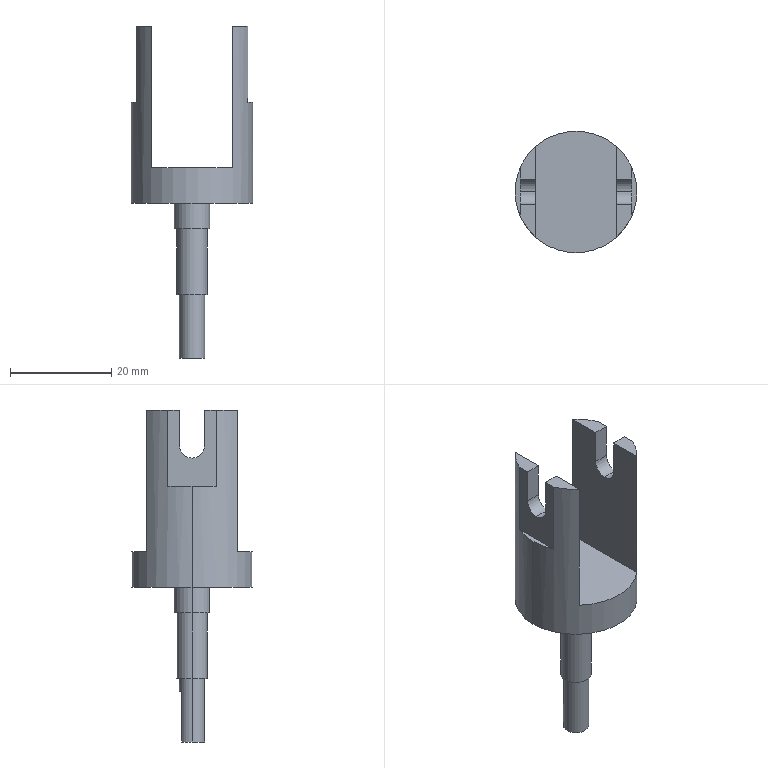Part | SolidWorks | features ICE 7, Extrusion 1 | 1 solid | 33 faces | box 24 x 24 x 65.5 mm | volume 6275 mm3 | plane 21 | cylinder 12 | commonest cylinder face diameters 5 x6 6 x2 7 x2 24 x2
STEP:
#1=CARTESIAN_POINT('',(-2.5,0.,-30.5));
#2=VERTEX_POINT('',#1);
#3=CARTESIAN_POINT('',(-1.5,2.,-30.5));
#4=VERTEX_POINT('',#3);
#5=CARTESIAN_POINT('',(0.,0.,-30.5));
#6=DIRECTION('',(0.,0.,-1.));
#7=DIRECTION('',(-1.,0.,0.));
#8=AXIS2_PLACEMENT_3D('',#5,#6,#7);
#9=CIRCLE('',#8,2.5);
#10=EDGE_CURVE('',#2,#4,#9,.T.);
#11=ORIENTED_EDGE('',*,*,#10,.F.);
#12=CARTESIAN_POINT('',(-2.5,0.,-18.));
#13=VERTEX_POINT('',#12);
#14=CARTESIAN_POINT('',(-2.5,0.,-30.5));
#15=DIRECTION('',(0.,0.,1.));
#16=VECTOR('',#15,1000.);
#17=LINE('',#14,#16);
#18=EDGE_CURVE('',#2,#13,#17,.T.);
#19=ORIENTED_EDGE('',*,*,#18,.T.);
#20=CARTESIAN_POINT('',(2.5,0.,-18.));
#21=VERTEX_POINT('',#20);
#22=CARTESIAN_POINT('',(0.,0.,-18.));
#23=DIRECTION('',(0.,0.,-1.));
#24=DIRECTION('',(-1.,0.,0.));
#25=AXIS2_PLACEMENT_3D('',#22,#23,#24);
#26=CIRCLE('',#25,2.5);
#27=EDGE_CURVE('',#13,#21,#26,.T.);
#28=ORIENTED_EDGE('',*,*,#27,.T.);
#29=CARTESIAN_POINT('',(2.5,0.,-30.5));
#30=VERTEX_POINT('',#29);
#31=CARTESIAN_POINT('',(2.5,0.,-30.5));
#32=DIRECTION('',(0.,0.,1.));
#33=VECTOR('',#32,1000.);
#34=LINE('',#31,#33);
#35=EDGE_CURVE('',#30,#21,#34,.T.);
#36=ORIENTED_EDGE('',*,*,#35,.F.);
#37=CARTESIAN_POINT('',(1.5,2.,-30.5));
#38=VERTEX_POINT('',#37);
#39=CARTESIAN_POINT('',(0.,0.,-30.5));
#40=DIRECTION('',(0.,0.,-1.));
#41=DIRECTION('',(-1.,0.,0.));
#42=AXIS2_PLACEMENT_3D('',#39,#40,#41);
#43=CIRCLE('',#42,2.5);
#44=EDGE_CURVE('',#38,#30,#43,.T.);
#45=ORIENTED_EDGE('',*,*,#44,.F.);
#46=CARTESIAN_POINT('',(1.5,2.,-20.5));
#47=VERTEX_POINT('',#46);
#48=CARTESIAN_POINT('',(1.5,2.,-30.5));
#49=DIRECTION('',(0.,0.,1.));
#50=VECTOR('',#49,1000.);
#51=LINE('',#48,#50);
#52=EDGE_CURVE('',#38,#47,#51,.T.);
#53=ORIENTED_EDGE('',*,*,#52,.T.);
#54=CARTESIAN_POINT('',(-1.5,2.,-20.5));
#55=VERTEX_POINT('',#54);
#56=CARTESIAN_POINT('',(0.,0.,-20.5));
#57=DIRECTION('',(0.,0.,1.));
#58=DIRECTION('',(1.,0.,0.));
#59=AXIS2_PLACEMENT_3D('',#56,#57,#58);
#60=CIRCLE('',#59,2.5);
#61=EDGE_CURVE('',#47,#55,#60,.T.);
#62=ORIENTED_EDGE('',*,*,#61,.T.);
#63=CARTESIAN_POINT('',(-1.5,2.,-30.5));
#64=DIRECTION('',(0.,0.,-1.));
#65=VECTOR('',#64,1000.);
#66=LINE('',#63,#65);
#67=EDGE_CURVE('',#55,#4,#66,.T.);
#68=ORIENTED_EDGE('',*,*,#67,.T.);
#69=EDGE_LOOP('',(#11,#19,#28,#36,#45,#53,#62,#68));
#70=FACE_OUTER_BOUND('',#69,.T.);
#71=CARTESIAN_POINT('',(0.,0.,-30.5));
#72=DIRECTION('',(0.,0.,1.));
#73=DIRECTION('',(1.,0.,0.));
#74=AXIS2_PLACEMENT_3D('',#71,#72,#73);
#75=CYLINDRICAL_SURFACE('',#74,2.5);
#76=ADVANCED_FACE('',(#70),#75,.T.);
#77=CARTESIAN_POINT('',(-3.,0.,-18.));
#78=VERTEX_POINT('',#77);
#79=CARTESIAN_POINT('',(3.,0.,-18.));
#80=VERTEX_POINT('',#79);
#81=CARTESIAN_POINT('',(0.,0.,-18.));
#82=DIRECTION('',(0.,0.,-1.));
#83=DIRECTION('',(-1.,0.,0.));
#84=AXIS2_PLACEMENT_3D('',#81,#82,#83);
#85=CIRCLE('',#84,3.);
#86=EDGE_CURVE('',#78,#80,#85,.T.);
#87=ORIENTED_EDGE('',*,*,#86,.F.);
#88=CARTESIAN_POINT('',(-3.,0.,-5.));
#89=VERTEX_POINT('',#88);
#90=CARTESIAN_POINT('',(-3.,0.,-18.));
#91=DIRECTION('',(0.,0.,1.));
#92=VECTOR('',#91,1000.);
#93=LINE('',#90,#92);
#94=EDGE_CURVE('',#78,#89,#93,.T.);
#95=ORIENTED_EDGE('',*,*,#94,.T.);
#96=CARTESIAN_POINT('',(3.,0.,-5.));
#97=VERTEX_POINT('',#96);
#98=CARTESIAN_POINT('',(0.,0.,-5.));
#99=DIRECTION('',(0.,0.,-1.));
#100=DIRECTION('',(-1.,0.,0.));
#101=AXIS2_PLACEMENT_3D('',#98,#99,#100);
#102=CIRCLE('',#101,3.);
#103=EDGE_CURVE('',#89,#97,#102,.T.);
#104=ORIENTED_EDGE('',*,*,#103,.T.);
#105=CARTESIAN_POINT('',(3.,0.,-18.));
#106=DIRECTION('',(0.,0.,1.));
#107=VECTOR('',#106,1000.);
#108=LINE('',#105,#107);
#109=EDGE_CURVE('',#80,#97,#108,.T.);
#110=ORIENTED_EDGE('',*,*,#109,.F.);
#111=EDGE_LOOP('',(#87,#95,#104,#110));
#112=FACE_OUTER_BOUND('',#111,.T.);
#113=CARTESIAN_POINT('',(0.,0.,-18.));
#114=DIRECTION('',(0.,0.,1.));
#115=DIRECTION('',(1.,0.,0.));
#116=AXIS2_PLACEMENT_3D('',#113,#114,#115);
#117=CYLINDRICAL_SURFACE('',#116,3.);
#118=ADVANCED_FACE('',(#112),#117,.T.);
#119=CARTESIAN_POINT('',(8.,0.,25.5));
#120=VERTEX_POINT('',#119);
#121=CARTESIAN_POINT('',(8.,2.5,28.));
#122=VERTEX_POINT('',#121);
#123=CARTESIAN_POINT('',(8.,0.,28.));
#124=DIRECTION('',(1.,0.,0.));
#125=DIRECTION('',(0.,1.,0.));
#126=AXIS2_PLACEMENT_3D('',#123,#124,#125);
#127=CIRCLE('',#126,2.5);
#128=EDGE_CURVE('',#120,#122,#127,.T.);
#129=ORIENTED_EDGE('',*,*,#128,.F.);
#130=CARTESIAN_POINT('',(11.,0.,25.5));
#131=VERTEX_POINT('',#130);
#132=CARTESIAN_POINT('',(-15.,0.,25.5));
#133=DIRECTION('',(1.,0.,0.));
#134=VECTOR('',#133,1000.);
#135=LINE('',#132,#134);
#136=EDGE_CURVE('',#120,#131,#135,.T.);
#137=ORIENTED_EDGE('',*,*,#136,.T.);
#138=CARTESIAN_POINT('',(11.,2.5,28.));
#139=VERTEX_POINT('',#138);
#140=CARTESIAN_POINT('',(11.,0.,28.));
#141=DIRECTION('',(1.,0.,0.));
#142=DIRECTION('',(0.,0.,1.));
#143=AXIS2_PLACEMENT_3D('',#140,#141,#142);
#144=CIRCLE('',#143,2.5);
#145=EDGE_CURVE('',#131,#139,#144,.T.);
#146=ORIENTED_EDGE('',*,*,#145,.T.);
#147=CARTESIAN_POINT('',(-15.,2.5,28.));
#148=DIRECTION('',(1.,0.,0.));
#149=VECTOR('',#148,1000.);
#150=LINE('',#147,#149);
#151=EDGE_CURVE('',#122,#139,#150,.T.);
#152=ORIENTED_EDGE('',*,*,#151,.F.);
#153=EDGE_LOOP('',(#129,#137,#146,#152));
#154=FACE_OUTER_BOUND('',#153,.T.);
#155=CARTESIAN_POINT('',(-15.,0.,28.));
#156=DIRECTION('',(1.,0.,0.));
#157=DIRECTION('',(0.,0.,-1.));
#158=AXIS2_PLACEMENT_3D('',#155,#156,#157);
#159=CYLINDRICAL_SURFACE('',#158,2.5);
#160=ADVANCED_FACE('',(#154),#159,.F.);
#161=CARTESIAN_POINT('',(-11.,2.5,28.));
#162=VERTEX_POINT('',#161);
#163=CARTESIAN_POINT('',(-11.,0.,25.5));
#164=VERTEX_POINT('',#163);
#165=CARTESIAN_POINT('',(-11.,0.,28.));
#166=DIRECTION('',(-1.,0.,0.));
#167=DIRECTION('',(0.,0.,-1.));
#168=AXIS2_PLACEMENT_3D('',#165,#166,#167);
#169=CIRCLE('',#168,2.5);
#170=EDGE_CURVE('',#162,#164,#169,.T.);
#171=ORIENTED_EDGE('',*,*,#170,.T.);
#172=CARTESIAN_POINT('',(-8.,0.,25.5));
#173=VERTEX_POINT('',#172);
#174=CARTESIAN_POINT('',(-15.,0.,25.5));
#175=DIRECTION('',(1.,0.,0.));
#176=VECTOR('',#175,1000.);
#177=LINE('',#174,#176);
#178=EDGE_CURVE('',#164,#173,#177,.T.);
#179=ORIENTED_EDGE('',*,*,#178,.T.);
#180=CARTESIAN_POINT('',(-8.,2.5,28.));
#181=VERTEX_POINT('',#180);
#182=CARTESIAN_POINT('',(-8.,0.,28.));
#183=DIRECTION('',(-1.,0.,0.));
#184=DIRECTION('',(0.,-1.,0.));
#185=AXIS2_PLACEMENT_3D('',#182,#183,#184);
#186=CIRCLE('',#185,2.5);
#187=EDGE_CURVE('',#181,#173,#186,.T.);
#188=ORIENTED_EDGE('',*,*,#187,.F.);
#189=CARTESIAN_POINT('',(-15.,2.5,28.));
#190=DIRECTION('',(1.,0.,0.));
#191=VECTOR('',#190,1000.);
#192=LINE('',#189,#191);
#193=EDGE_CURVE('',#162,#181,#192,.T.);
#194=ORIENTED_EDGE('',*,*,#193,.F.);
#195=EDGE_LOOP('',(#171,#179,#188,#194));
#196=FACE_OUTER_BOUND('',#195,.T.);
#197=CARTESIAN_POINT('',(-15.,0.,28.));
#198=DIRECTION('',(1.,0.,0.));
#199=DIRECTION('',(0.,0.,-1.));
#200=AXIS2_PLACEMENT_3D('',#197,#198,#199);
#201=CYLINDRICAL_SURFACE('',#200,2.5);
#202=ADVANCED_FACE('',(#196),#201,.F.);
#203=CARTESIAN_POINT('',(-3.5,0.,-5.));
#204=VERTEX_POINT('',#203);
#205=CARTESIAN_POINT('',(3.5,0.,-5.));
#206=VERTEX_POINT('',#205);
#207=CARTESIAN_POINT('',(0.,0.,-5.));
#208=DIRECTION('',(0.,0.,-1.));
#209=DIRECTION('',(-1.,0.,0.));
#210=AXIS2_PLACEMENT_3D('',#207,#208,#209);
#211=CIRCLE('',#210,3.5);
#212=EDGE_CURVE('',#204,#206,#211,.T.);
#213=ORIENTED_EDGE('',*,*,#212,.F.);
#214=CARTESIAN_POINT('',(-3.5,0.,0.));
#215=VERTEX_POINT('',#214);
#216=CARTESIAN_POINT('',(-3.5,0.,-5.));
#217=DIRECTION('',(0.,0.,1.));
#218=VECTOR('',#217,1000.);
#219=LINE('',#216,#218);
#220=EDGE_CURVE('',#204,#215,#219,.T.);
#221=ORIENTED_EDGE('',*,*,#220,.T.);
#222=CARTESIAN_POINT('',(3.5,0.,0.));
#223=VERTEX_POINT('',#222);
#224=CARTESIAN_POINT('',(0.,0.,0.));
#225=DIRECTION('',(0.,0.,-1.));
#226=DIRECTION('',(-1.,0.,0.));
#227=AXIS2_PLACEMENT_3D('',#224,#225,#226);
#228=CIRCLE('',#227,3.5);
#229=EDGE_CURVE('',#215,#223,#228,.T.);
#230=ORIENTED_EDGE('',*,*,#229,.T.);
#231=CARTESIAN_POINT('',(3.5,0.,-5.));
#232=DIRECTION('',(0.,0.,1.));
#233=VECTOR('',#232,1000.);
#234=LINE('',#231,#233);
#235=EDGE_CURVE('',#206,#223,#234,.T.);
#236=ORIENTED_EDGE('',*,*,#235,.F.);
#237=EDGE_LOOP('',(#213,#221,#230,#236));
#238=FACE_OUTER_BOUND('',#237,.T.);
#239=CARTESIAN_POINT('',(0.,0.,-5.));
#240=DIRECTION('',(0.,0.,1.));
#241=DIRECTION('',(1.,0.,0.));
#242=AXIS2_PLACEMENT_3D('',#239,#240,#241);
#243=CYLINDRICAL_SURFACE('',#242,3.5);
#244=ADVANCED_FACE('',(#238),#243,.T.);
#245=CARTESIAN_POINT('',(12.,0.,20.));
#246=VERTEX_POINT('',#245);
#247=CARTESIAN_POINT('',(11.,4.796,20.));
#248=VERTEX_POINT('',#247);
#249=CARTESIAN_POINT('',(0.,0.,20.));
#250=DIRECTION('',(0.,0.,1.));
#251=DIRECTION('',(1.,0.,0.));
#252=AXIS2_PLACEMENT_3D('',#249,#250,#251);
#253=CIRCLE('',#252,12.);
#254=EDGE_CURVE('',#246,#248,#253,.T.);
#255=ORIENTED_EDGE('',*,*,#254,.F.);
#256=CARTESIAN_POINT('',(12.,0.,0.));
#257=VERTEX_POINT('',#256);
#258=CARTESIAN_POINT('',(12.,0.,35.));
#259=DIRECTION('',(0.,0.,-1.));
#260=VECTOR('',#259,1000.);
#261=LINE('',#258,#260);
#262=EDGE_CURVE('',#246,#257,#261,.T.);
#263=ORIENTED_EDGE('',*,*,#262,.T.);
#264=CARTESIAN_POINT('',(-12.,0.,0.));
#265=VERTEX_POINT('',#264);
#266=CARTESIAN_POINT('',(0.,0.,0.));
#267=DIRECTION('',(0.,0.,1.));
#268=DIRECTION('',(1.,0.,0.));
#269=AXIS2_PLACEMENT_3D('',#266,#267,#268);
#270=CIRCLE('',#269,12.);
#271=EDGE_CURVE('',#257,#265,#270,.T.);
#272=ORIENTED_EDGE('',*,*,#271,.T.);
#273=CARTESIAN_POINT('',(-12.,0.,20.));
#274=VERTEX_POINT('',#273);
#275=CARTESIAN_POINT('',(-12.,0.,35.));
#276=DIRECTION('',(0.,0.,-1.));
#277=VECTOR('',#276,1000.);
#278=LINE('',#275,#277);
#279=EDGE_CURVE('',#274,#265,#278,.T.);
#280=ORIENTED_EDGE('',*,*,#279,.F.);
#281=CARTESIAN_POINT('',(-11.,4.796,20.));
#282=VERTEX_POINT('',#281);
#283=CARTESIAN_POINT('',(0.,0.,20.));
#284=DIRECTION('',(0.,0.,1.));
#285=DIRECTION('',(-1.,0.,0.));
#286=AXIS2_PLACEMENT_3D('',#283,#284,#285);
#287=CIRCLE('',#286,12.);
#288=EDGE_CURVE('',#282,#274,#287,.T.);
#289=ORIENTED_EDGE('',*,*,#288,.F.);
#290=CARTESIAN_POINT('',(-11.,4.796,35.));
#291=VERTEX_POINT('',#290);
#292=CARTESIAN_POINT('',(-11.,4.796,20.));
#293=DIRECTION('',(0.,0.,1.));
#294=VECTOR('',#293,1000.);
#295=LINE('',#292,#294);
#296=EDGE_CURVE('',#282,#291,#295,.T.);
#297=ORIENTED_EDGE('',*,*,#296,.T.);
#298=CARTESIAN_POINT('',(-8.,8.944,35.));
#299=VERTEX_POINT('',#298);
#300=CARTESIAN_POINT('',(0.,0.,35.));
#301=DIRECTION('',(0.,0.,1.));
#302=DIRECTION('',(1.,0.,0.));
#303=AXIS2_PLACEMENT_3D('',#300,#301,#302);
#304=CIRCLE('',#303,12.);
#305=EDGE_CURVE('',#299,#291,#304,.T.);
#306=ORIENTED_EDGE('',*,*,#305,.F.);
#307=CARTESIAN_POINT('',(-8.,8.944,7.));
#308=VERTEX_POINT('',#307);
#309=CARTESIAN_POINT('',(-8.,8.944,35.));
#310=DIRECTION('',(0.,0.,-1.));
#311=VECTOR('',#310,1000.);
#312=LINE('',#309,#311);
#313=EDGE_CURVE('',#299,#308,#312,.T.);
#314=ORIENTED_EDGE('',*,*,#313,.T.);
#315=CARTESIAN_POINT('',(8.,8.944,7.));
#316=VERTEX_POINT('',#315);
#317=CARTESIAN_POINT('',(0.,0.,7.));
#318=DIRECTION('',(0.,0.,1.));
#319=DIRECTION('',(1.,0.,0.));
#320=AXIS2_PLACEMENT_3D('',#317,#318,#319);
#321=CIRCLE('',#320,12.);
#322=EDGE_CURVE('',#316,#308,#321,.T.);
#323=ORIENTED_EDGE('',*,*,#322,.F.);
#324=CARTESIAN_POINT('',(8.,8.944,35.));
#325=VERTEX_POINT('',#324);
#326=CARTESIAN_POINT('',(8.,8.944,35.));
#327=DIRECTION('',(0.,0.,1.));
#328=VECTOR('',#327,1000.);
#329=LINE('',#326,#328);
#330=EDGE_CURVE('',#316,#325,#329,.T.);
#331=ORIENTED_EDGE('',*,*,#330,.T.);
#332=CARTESIAN_POINT('',(11.,4.796,35.));
#333=VERTEX_POINT('',#332);
#334=CARTESIAN_POINT('',(0.,0.,35.));
#335=DIRECTION('',(0.,0.,1.));
#336=DIRECTION('',(1.,0.,0.));
#337=AXIS2_PLACEMENT_3D('',#334,#335,#336);
#338=CIRCLE('',#337,12.);
#339=EDGE_CURVE('',#333,#325,#338,.T.);
#340=ORIENTED_EDGE('',*,*,#339,.F.);
#341=CARTESIAN_POINT('',(11.,4.796,20.));
#342=DIRECTION('',(0.,0.,1.));
#343=VECTOR('',#342,1000.);
#344=LINE('',#341,#343);
#345=EDGE_CURVE('',#248,#333,#344,.T.);
#346=ORIENTED_EDGE('',*,*,#345,.F.);
#347=EDGE_LOOP('',(#255,#263,#272,#280,#289,#297,#306,#314,#323,#331,#340,#346));
#348=FACE_OUTER_BOUND('',#347,.T.);
#349=CARTESIAN_POINT('',(0.,0.,35.));
#350=DIRECTION('',(0.,0.,-1.));
#351=DIRECTION('',(-1.,0.,0.));
#352=AXIS2_PLACEMENT_3D('',#349,#350,#351);
#353=CYLINDRICAL_SURFACE('',#352,12.);
#354=ADVANCED_FACE('',(#348),#353,.T.);
#355=CARTESIAN_POINT('',(11.,-2.5,35.));
#356=VERTEX_POINT('',#355);
#357=CARTESIAN_POINT('',(11.,-4.796,35.));
#358=VERTEX_POINT('',#357);
#359=CARTESIAN_POINT('',(11.,-4.796,35.));
#360=DIRECTION('',(0.,-1.,0.));
#361=VECTOR('',#360,1000.);
#362=LINE('',#359,#361);
#363=EDGE_CURVE('',#356,#358,#362,.T.);
#364=ORIENTED_EDGE('',*,*,#363,.F.);
#365=CARTESIAN_POINT('',(8.,-2.5,35.));
#366=VERTEX_POINT('',#365);
#367=CARTESIAN_POINT('',(-15.,-2.5,35.));
#368=DIRECTION('',(1.,0.,0.));
#369=VECTOR('',#368,1000.);
#370=LINE('',#367,#369);
#371=EDGE_CURVE('',#366,#356,#370,.T.);
#372=ORIENTED_EDGE('',*,*,#371,.F.);
#373=CARTESIAN_POINT('',(8.,-8.944,35.));
#374=VERTEX_POINT('',#373);
#375=CARTESIAN_POINT('',(8.,0.,35.));
#376=DIRECTION('',(0.,1.,0.));
#377=VECTOR('',#376,1000.);
#378=LINE('',#375,#377);
#379=EDGE_CURVE('',#374,#366,#378,.T.);
#380=ORIENTED_EDGE('',*,*,#379,.F.);
#381=CARTESIAN_POINT('',(0.,0.,35.));
#382=DIRECTION('',(0.,0.,1.));
#383=DIRECTION('',(1.,0.,0.));
#384=AXIS2_PLACEMENT_3D('',#381,#382,#383);
#385=CIRCLE('',#384,12.);
#386=EDGE_CURVE('',#374,#358,#385,.T.);
#387=ORIENTED_EDGE('',*,*,#386,.T.);
#388=EDGE_LOOP('',(#364,#372,#380,#387));
#389=FACE_OUTER_BOUND('',#388,.T.);
#390=CARTESIAN_POINT('',(0.,0.,35.));
#391=DIRECTION('',(0.,0.,1.));
#392=DIRECTION('',(1.,0.,0.));
#393=AXIS2_PLACEMENT_3D('',#390,#391,#392);
#394=PLANE('',#393);
#395=ADVANCED_FACE('',(#389),#394,.T.);
#396=CARTESIAN_POINT('',(-11.,-4.796,35.));
#397=VERTEX_POINT('',#396);
#398=CARTESIAN_POINT('',(-11.,-2.5,35.));
#399=VERTEX_POINT('',#398);
#400=CARTESIAN_POINT('',(-11.,-4.796,35.));
#401=DIRECTION('',(0.,1.,0.));
#402=VECTOR('',#401,1000.);
#403=LINE('',#400,#402);
#404=EDGE_CURVE('',#397,#399,#403,.T.);
#405=ORIENTED_EDGE('',*,*,#404,.F.);
#406=CARTESIAN_POINT('',(-8.,-8.944,35.));
#407=VERTEX_POINT('',#406);
#408=CARTESIAN_POINT('',(0.,0.,35.));
#409=DIRECTION('',(0.,0.,1.));
#410=DIRECTION('',(1.,0.,0.));
#411=AXIS2_PLACEMENT_3D('',#408,#409,#410);
#412=CIRCLE('',#411,12.);
#413=EDGE_CURVE('',#397,#407,#412,.T.);
#414=ORIENTED_EDGE('',*,*,#413,.T.);
#415=CARTESIAN_POINT('',(-8.,-2.5,35.));
#416=VERTEX_POINT('',#415);
#417=CARTESIAN_POINT('',(-8.,0.,35.));
#418=DIRECTION('',(0.,-1.,0.));
#419=VECTOR('',#418,1000.);
#420=LINE('',#417,#419);
#421=EDGE_CURVE('',#416,#407,#420,.T.);
#422=ORIENTED_EDGE('',*,*,#421,.F.);
#423=CARTESIAN_POINT('',(-15.,-2.5,35.));
#424=DIRECTION('',(1.,0.,0.));
#425=VECTOR('',#424,1000.);
#426=LINE('',#423,#425);
#427=EDGE_CURVE('',#399,#416,#426,.T.);
#428=ORIENTED_EDGE('',*,*,#427,.F.);
#429=EDGE_LOOP('',(#405,#414,#422,#428));
#430=FACE_OUTER_BOUND('',#429,.T.);
#431=CARTESIAN_POINT('',(0.,0.,35.));
#432=DIRECTION('',(0.,0.,1.));
#433=DIRECTION('',(1.,0.,0.));
#434=AXIS2_PLACEMENT_3D('',#431,#432,#433);
#435=PLANE('',#434);
#436=ADVANCED_FACE('',(#430),#435,.T.);
#437=CARTESIAN_POINT('',(11.,2.5,35.));
#438=VERTEX_POINT('',#437);
#439=CARTESIAN_POINT('',(11.,-4.796,35.));
#440=DIRECTION('',(0.,-1.,0.));
#441=VECTOR('',#440,1000.);
#442=LINE('',#439,#441);
#443=EDGE_CURVE('',#333,#438,#442,.T.);
#444=ORIENTED_EDGE('',*,*,#443,.F.);
#445=ORIENTED_EDGE('',*,*,#339,.T.);
#446=CARTESIAN_POINT('',(8.,2.5,35.));
#447=VERTEX_POINT('',#446);
#448=CARTESIAN_POINT('',(8.,0.,35.));
#449=DIRECTION('',(0.,1.,0.));
#450=VECTOR('',#449,1000.);
#451=LINE('',#448,#450);
#452=EDGE_CURVE('',#447,#325,#451,.T.);
#453=ORIENTED_EDGE('',*,*,#452,.F.);
#454=CARTESIAN_POINT('',(-15.,2.5,35.));
#455=DIRECTION('',(1.,0.,0.));
#456=VECTOR('',#455,1000.);
#457=LINE('',#454,#456);
#458=EDGE_CURVE('',#447,#438,#457,.T.);
#459=ORIENTED_EDGE('',*,*,#458,.T.);
#460=EDGE_LOOP('',(#444,#445,#453,#459));
#461=FACE_OUTER_BOUND('',#460,.T.);
#462=CARTESIAN_POINT('',(0.,0.,35.));
#463=DIRECTION('',(0.,0.,1.));
#464=DIRECTION('',(1.,0.,0.));
#465=AXIS2_PLACEMENT_3D('',#462,#463,#464);
#466=PLANE('',#465);
#467=ADVANCED_FACE('',(#461),#466,.T.);
#468=ORIENTED_EDGE('',*,*,#262,.F.);
#469=CARTESIAN_POINT('',(11.,-4.796,20.));
#470=VERTEX_POINT('',#469);
#471=CARTESIAN_POINT('',(0.,0.,20.));
#472=DIRECTION('',(0.,0.,1.));
#473=DIRECTION('',(1.,0.,0.));
#474=AXIS2_PLACEMENT_3D('',#471,#472,#473);
#475=CIRCLE('',#474,12.);
#476=EDGE_CURVE('',#470,#246,#475,.T.);
#477=ORIENTED_EDGE('',*,*,#476,.F.);
#478=CARTESIAN_POINT('',(11.,-4.796,20.));
#479=DIRECTION('',(0.,0.,1.));
#480=VECTOR('',#479,1000.);
#481=LINE('',#478,#480);
#482=EDGE_CURVE('',#470,#358,#481,.T.);
#483=ORIENTED_EDGE('',*,*,#482,.T.);
#484=ORIENTED_EDGE('',*,*,#386,.F.);
#485=CARTESIAN_POINT('',(8.,-8.944,7.));
#486=VERTEX_POINT('',#485);
#487=CARTESIAN_POINT('',(8.,-8.944,35.));
#488=DIRECTION('',(0.,0.,-1.));
#489=VECTOR('',#488,1000.);
#490=LINE('',#487,#489);
#491=EDGE_CURVE('',#374,#486,#490,.T.);
#492=ORIENTED_EDGE('',*,*,#491,.T.);
#493=CARTESIAN_POINT('',(-8.,-8.944,7.));
#494=VERTEX_POINT('',#493);
#495=CARTESIAN_POINT('',(0.,0.,7.));
#496=DIRECTION('',(0.,0.,1.));
#497=DIRECTION('',(1.,0.,0.));
#498=AXIS2_PLACEMENT_3D('',#495,#496,#497);
#499=CIRCLE('',#498,12.);
#500=EDGE_CURVE('',#494,#486,#499,.T.);
#501=ORIENTED_EDGE('',*,*,#500,.F.);
#502=CARTESIAN_POINT('',(-8.,-8.944,35.));
#503=DIRECTION('',(0.,0.,1.));
#504=VECTOR('',#503,1000.);
#505=LINE('',#502,#504);
#506=EDGE_CURVE('',#494,#407,#505,.T.);
#507=ORIENTED_EDGE('',*,*,#506,.T.);
#508=ORIENTED_EDGE('',*,*,#413,.F.);
#509=CARTESIAN_POINT('',(-11.,-4.796,20.));
#510=VERTEX_POINT('',#509);
#511=CARTESIAN_POINT('',(-11.,-4.796,20.));
#512=DIRECTION('',(0.,0.,1.));
#513=VECTOR('',#512,1000.);
#514=LINE('',#511,#513);
#515=EDGE_CURVE('',#510,#397,#514,.T.);
#516=ORIENTED_EDGE('',*,*,#515,.F.);
#517=CARTESIAN_POINT('',(0.,0.,20.));
#518=DIRECTION('',(0.,0.,1.));
#519=DIRECTION('',(-1.,0.,0.));
#520=AXIS2_PLACEMENT_3D('',#517,#518,#519);
#521=CIRCLE('',#520,12.);
#522=EDGE_CURVE('',#274,#510,#521,.T.);
#523=ORIENTED_EDGE('',*,*,#522,.F.);
#524=ORIENTED_EDGE('',*,*,#279,.T.);
#525=CARTESIAN_POINT('',(0.,0.,0.));
#526=DIRECTION('',(0.,0.,1.));
#527=DIRECTION('',(1.,0.,0.));
#528=AXIS2_PLACEMENT_3D('',#525,#526,#527);
#529=CIRCLE('',#528,12.);
#530=EDGE_CURVE('',#265,#257,#529,.T.);
#531=ORIENTED_EDGE('',*,*,#530,.T.);
#532=EDGE_LOOP('',(#468,#477,#483,#484,#492,#501,#507,#508,#516,#523,#524,#531));
#533=FACE_OUTER_BOUND('',#532,.T.);
#534=CARTESIAN_POINT('',(0.,0.,35.));
#535=DIRECTION('',(0.,0.,-1.));
#536=DIRECTION('',(-1.,0.,0.));
#537=AXIS2_PLACEMENT_3D('',#534,#535,#536);
#538=CYLINDRICAL_SURFACE('',#537,12.);
#539=ADVANCED_FACE('',(#533),#538,.T.);
#540=CARTESIAN_POINT('',(-11.,2.5,35.));
#541=VERTEX_POINT('',#540);
#542=CARTESIAN_POINT('',(-11.,-4.796,35.));
#543=DIRECTION('',(0.,1.,0.));
#544=VECTOR('',#543,1000.);
#545=LINE('',#542,#544);
#546=EDGE_CURVE('',#541,#291,#545,.T.);
#547=ORIENTED_EDGE('',*,*,#546,.F.);
#548=CARTESIAN_POINT('',(-8.,2.5,35.));
#549=VERTEX_POINT('',#548);
#550=CARTESIAN_POINT('',(-15.,2.5,35.));
#551=DIRECTION('',(1.,0.,0.));
#552=VECTOR('',#551,1000.);
#553=LINE('',#550,#552);
#554=EDGE_CURVE('',#541,#549,#553,.T.);
#555=ORIENTED_EDGE('',*,*,#554,.T.);
#556=CARTESIAN_POINT('',(-8.,0.,35.));
#557=DIRECTION('',(0.,-1.,0.));
#558=VECTOR('',#557,1000.);
#559=LINE('',#556,#558);
#560=EDGE_CURVE('',#299,#549,#559,.T.);
#561=ORIENTED_EDGE('',*,*,#560,.F.);
#562=ORIENTED_EDGE('',*,*,#305,.T.);
#563=EDGE_LOOP('',(#547,#555,#561,#562));
#564=FACE_OUTER_BOUND('',#563,.T.);
#565=CARTESIAN_POINT('',(0.,0.,35.));
#566=DIRECTION('',(0.,0.,1.));
#567=DIRECTION('',(1.,0.,0.));
#568=AXIS2_PLACEMENT_3D('',#565,#566,#567);
#569=PLANE('',#568);
#570=ADVANCED_FACE('',(#564),#569,.T.);
#571=CARTESIAN_POINT('',(0.,0.,0.));
#572=DIRECTION('',(0.,0.,-1.));
#573=DIRECTION('',(-1.,0.,0.));
#574=AXIS2_PLACEMENT_3D('',#571,#572,#573);
#575=CIRCLE('',#574,3.5);
#576=EDGE_CURVE('',#223,#215,#575,.T.);
#577=ORIENTED_EDGE('',*,*,#576,.F.);
#578=ORIENTED_EDGE('',*,*,#229,.F.);
#579=EDGE_LOOP('',(#577,#578));
#580=FACE_BOUND('',#579,.T.);
#581=ORIENTED_EDGE('',*,*,#530,.F.);
#582=ORIENTED_EDGE('',*,*,#271,.F.);
#583=EDGE_LOOP('',(#581,#582));
#584=FACE_OUTER_BOUND('',#583,.T.);
#585=CARTESIAN_POINT('',(0.,0.,0.));
#586=DIRECTION('',(0.,0.,1.));
#587=DIRECTION('',(1.,0.,0.));
#588=AXIS2_PLACEMENT_3D('',#585,#586,#587);
#589=PLANE('',#588);
#590=ADVANCED_FACE('',(#580,#584),#589,.F.);
#591=ORIENTED_EDGE('',*,*,#220,.F.);
#592=CARTESIAN_POINT('',(0.,0.,-5.));
#593=DIRECTION('',(0.,0.,-1.));
#594=DIRECTION('',(-1.,0.,0.));
#595=AXIS2_PLACEMENT_3D('',#592,#593,#594);
#596=CIRCLE('',#595,3.5);
#597=EDGE_CURVE('',#206,#204,#596,.T.);
#598=ORIENTED_EDGE('',*,*,#597,.F.);
#599=ORIENTED_EDGE('',*,*,#235,.T.);
#600=ORIENTED_EDGE('',*,*,#576,.T.);
#601=EDGE_LOOP('',(#591,#598,#599,#600));
#602=FACE_OUTER_BOUND('',#601,.T.);
#603=CARTESIAN_POINT('',(0.,0.,-5.));
#604=DIRECTION('',(0.,0.,1.));
#605=DIRECTION('',(1.,0.,0.));
#606=AXIS2_PLACEMENT_3D('',#603,#604,#605);
#607=CYLINDRICAL_SURFACE('',#606,3.5);
#608=ADVANCED_FACE('',(#602),#607,.T.);
#609=CARTESIAN_POINT('',(0.,0.,-5.));
#610=DIRECTION('',(0.,0.,-1.));
#611=DIRECTION('',(-1.,0.,0.));
#612=AXIS2_PLACEMENT_3D('',#609,#610,#611);
#613=CIRCLE('',#612,3.);
#614=EDGE_CURVE('',#97,#89,#613,.T.);
#615=ORIENTED_EDGE('',*,*,#614,.F.);
#616=ORIENTED_EDGE('',*,*,#103,.F.);
#617=EDGE_LOOP('',(#615,#616));
#618=FACE_BOUND('',#617,.T.);
#619=ORIENTED_EDGE('',*,*,#597,.T.);
#620=ORIENTED_EDGE('',*,*,#212,.T.);
#621=EDGE_LOOP('',(#619,#620));
#622=FACE_OUTER_BOUND('',#621,.T.);
#623=CARTESIAN_POINT('',(0.,0.,-5.));
#624=DIRECTION('',(0.,0.,-1.));
#625=DIRECTION('',(-1.,0.,0.));
#626=AXIS2_PLACEMENT_3D('',#623,#624,#625);
#627=PLANE('',#626);
#628=ADVANCED_FACE('',(#618,#622),#627,.T.);
#629=ORIENTED_EDGE('',*,*,#322,.T.);
#630=CARTESIAN_POINT('',(-8.,12.5,7.));
#631=DIRECTION('',(0.,-1.,0.));
#632=VECTOR('',#631,1000.);
#633=LINE('',#630,#632);
#634=EDGE_CURVE('',#308,#494,#633,.T.);
#635=ORIENTED_EDGE('',*,*,#634,.T.);
#636=ORIENTED_EDGE('',*,*,#500,.T.);
#637=CARTESIAN_POINT('',(8.,12.5,7.));
#638=DIRECTION('',(0.,1.,0.));
#639=VECTOR('',#638,1000.);
#640=LINE('',#637,#639);
#641=EDGE_CURVE('',#486,#316,#640,.T.);
#642=ORIENTED_EDGE('',*,*,#641,.T.);
#643=EDGE_LOOP('',(#629,#635,#636,#642));
#644=FACE_OUTER_BOUND('',#643,.T.);
#645=CARTESIAN_POINT('',(0.,0.,7.));
#646=DIRECTION('',(0.,0.,1.));
#647=DIRECTION('',(1.,0.,0.));
#648=AXIS2_PLACEMENT_3D('',#645,#646,#647);
#649=PLANE('',#648);
#650=ADVANCED_FACE('',(#644),#649,.T.);
#651=ORIENTED_EDGE('',*,*,#379,.T.);
#652=CARTESIAN_POINT('',(8.,-2.5,28.));
#653=VERTEX_POINT('',#652);
#654=CARTESIAN_POINT('',(8.,-2.5,7.));
#655=DIRECTION('',(0.,0.,-1.));
#656=VECTOR('',#655,1000.);
#657=LINE('',#654,#656);
#658=EDGE_CURVE('',#366,#653,#657,.T.);
#659=ORIENTED_EDGE('',*,*,#658,.T.);
#660=CARTESIAN_POINT('',(8.,0.,28.));
#661=DIRECTION('',(1.,0.,0.));
#662=DIRECTION('',(0.,1.,0.));
#663=AXIS2_PLACEMENT_3D('',#660,#661,#662);
#664=CIRCLE('',#663,2.5);
#665=EDGE_CURVE('',#653,#120,#664,.T.);
#666=ORIENTED_EDGE('',*,*,#665,.T.);
#667=ORIENTED_EDGE('',*,*,#128,.T.);
#668=CARTESIAN_POINT('',(8.,2.5,7.));
#669=DIRECTION('',(0.,0.,1.));
#670=VECTOR('',#669,1000.);
#671=LINE('',#668,#670);
#672=EDGE_CURVE('',#122,#447,#671,.T.);
#673=ORIENTED_EDGE('',*,*,#672,.T.);
#674=ORIENTED_EDGE('',*,*,#452,.T.);
#675=ORIENTED_EDGE('',*,*,#330,.F.);
#676=ORIENTED_EDGE('',*,*,#641,.F.);
#677=ORIENTED_EDGE('',*,*,#491,.F.);
#678=EDGE_LOOP('',(#651,#659,#666,#667,#673,#674,#675,#676,#677));
#679=FACE_OUTER_BOUND('',#678,.T.);
#680=CARTESIAN_POINT('',(8.,12.5,7.));
#681=DIRECTION('',(1.,0.,0.));
#682=DIRECTION('',(0.,1.,0.));
#683=AXIS2_PLACEMENT_3D('',#680,#681,#682);
#684=PLANE('',#683);
#685=ADVANCED_FACE('',(#679),#684,.F.);
#686=ORIENTED_EDGE('',*,*,#187,.T.);
#687=CARTESIAN_POINT('',(-8.,-2.5,28.));
#688=VERTEX_POINT('',#687);
#689=CARTESIAN_POINT('',(-8.,0.,28.));
#690=DIRECTION('',(-1.,0.,0.));
#691=DIRECTION('',(0.,-1.,0.));
#692=AXIS2_PLACEMENT_3D('',#689,#690,#691);
#693=CIRCLE('',#692,2.5);
#694=EDGE_CURVE('',#173,#688,#693,.T.);
#695=ORIENTED_EDGE('',*,*,#694,.T.);
#696=CARTESIAN_POINT('',(-8.,-2.5,7.));
#697=DIRECTION('',(0.,0.,1.));
#698=VECTOR('',#697,1000.);
#699=LINE('',#696,#698);
#700=EDGE_CURVE('',#688,#416,#699,.T.);
#701=ORIENTED_EDGE('',*,*,#700,.T.);
#702=ORIENTED_EDGE('',*,*,#421,.T.);
#703=ORIENTED_EDGE('',*,*,#506,.F.);
#704=ORIENTED_EDGE('',*,*,#634,.F.);
#705=ORIENTED_EDGE('',*,*,#313,.F.);
#706=ORIENTED_EDGE('',*,*,#560,.T.);
#707=CARTESIAN_POINT('',(-8.,2.5,7.));
#708=DIRECTION('',(0.,0.,-1.));
#709=VECTOR('',#708,1000.);
#710=LINE('',#707,#709);
#711=EDGE_CURVE('',#549,#181,#710,.T.);
#712=ORIENTED_EDGE('',*,*,#711,.T.);
#713=EDGE_LOOP('',(#686,#695,#701,#702,#703,#704,#705,#706,#712));
#714=FACE_OUTER_BOUND('',#713,.T.);
#715=CARTESIAN_POINT('',(-8.,12.5,7.));
#716=DIRECTION('',(-1.,0.,0.));
#717=DIRECTION('',(0.,-1.,0.));
#718=AXIS2_PLACEMENT_3D('',#715,#716,#717);
#719=PLANE('',#718);
#720=ADVANCED_FACE('',(#714),#719,.F.);
#721=ORIENTED_EDGE('',*,*,#554,.F.);
#722=CARTESIAN_POINT('',(-11.,2.5,35.));
#723=DIRECTION('',(0.,0.,-1.));
#724=VECTOR('',#723,1000.);
#725=LINE('',#722,#724);
#726=EDGE_CURVE('',#541,#162,#725,.T.);
#727=ORIENTED_EDGE('',*,*,#726,.T.);
#728=ORIENTED_EDGE('',*,*,#193,.T.);
#729=ORIENTED_EDGE('',*,*,#711,.F.);
#730=EDGE_LOOP('',(#721,#727,#728,#729));
#731=FACE_OUTER_BOUND('',#730,.T.);
#732=CARTESIAN_POINT('',(-15.,2.5,35.));
#733=DIRECTION('',(0.,1.,0.));
#734=DIRECTION('',(0.,0.,1.));
#735=AXIS2_PLACEMENT_3D('',#732,#733,#734);
#736=PLANE('',#735);
#737=ADVANCED_FACE('',(#731),#736,.F.);
#738=CARTESIAN_POINT('',(-11.,-2.5,28.));
#739=VERTEX_POINT('',#738);
#740=CARTESIAN_POINT('',(-15.,-2.5,28.));
#741=DIRECTION('',(1.,0.,0.));
#742=VECTOR('',#741,1000.);
#743=LINE('',#740,#742);
#744=EDGE_CURVE('',#739,#688,#743,.T.);
#745=ORIENTED_EDGE('',*,*,#744,.F.);
#746=CARTESIAN_POINT('',(-11.,-2.5,28.));
#747=DIRECTION('',(0.,0.,1.));
#748=VECTOR('',#747,1000.);
#749=LINE('',#746,#748);
#750=EDGE_CURVE('',#739,#399,#749,.T.);
#751=ORIENTED_EDGE('',*,*,#750,.T.);
#752=ORIENTED_EDGE('',*,*,#427,.T.);
#753=ORIENTED_EDGE('',*,*,#700,.F.);
#754=EDGE_LOOP('',(#745,#751,#752,#753));
#755=FACE_OUTER_BOUND('',#754,.T.);
#756=CARTESIAN_POINT('',(-15.,-2.5,28.));
#757=DIRECTION('',(0.,-1.,0.));
#758=DIRECTION('',(0.,0.,-1.));
#759=AXIS2_PLACEMENT_3D('',#756,#757,#758);
#760=PLANE('',#759);
#761=ADVANCED_FACE('',(#755),#760,.F.);
#762=ORIENTED_EDGE('',*,*,#178,.F.);
#763=CARTESIAN_POINT('',(-11.,0.,28.));
#764=DIRECTION('',(-1.,0.,0.));
#765=DIRECTION('',(0.,0.,-1.));
#766=AXIS2_PLACEMENT_3D('',#763,#764,#765);
#767=CIRCLE('',#766,2.5);
#768=EDGE_CURVE('',#164,#739,#767,.T.);
#769=ORIENTED_EDGE('',*,*,#768,.T.);
#770=ORIENTED_EDGE('',*,*,#744,.T.);
#771=ORIENTED_EDGE('',*,*,#694,.F.);
#772=EDGE_LOOP('',(#762,#769,#770,#771));
#773=FACE_OUTER_BOUND('',#772,.T.);
#774=CARTESIAN_POINT('',(-15.,0.,28.));
#775=DIRECTION('',(1.,0.,0.));
#776=DIRECTION('',(0.,0.,-1.));
#777=AXIS2_PLACEMENT_3D('',#774,#775,#776);
#778=CYLINDRICAL_SURFACE('',#777,2.5);
#779=ADVANCED_FACE('',(#773),#778,.F.);
#780=ORIENTED_EDGE('',*,*,#136,.F.);
#781=ORIENTED_EDGE('',*,*,#665,.F.);
#782=CARTESIAN_POINT('',(11.,-2.5,28.));
#783=VERTEX_POINT('',#782);
#784=CARTESIAN_POINT('',(-15.,-2.5,28.));
#785=DIRECTION('',(1.,0.,0.));
#786=VECTOR('',#785,1000.);
#787=LINE('',#784,#786);
#788=EDGE_CURVE('',#653,#783,#787,.T.);
#789=ORIENTED_EDGE('',*,*,#788,.T.);
#790=CARTESIAN_POINT('',(11.,0.,28.));
#791=DIRECTION('',(1.,0.,0.));
#792=DIRECTION('',(0.,0.,1.));
#793=AXIS2_PLACEMENT_3D('',#790,#791,#792);
#794=CIRCLE('',#793,2.5);
#795=EDGE_CURVE('',#783,#131,#794,.T.);
#796=ORIENTED_EDGE('',*,*,#795,.T.);
#797=EDGE_LOOP('',(#780,#781,#789,#796));
#798=FACE_OUTER_BOUND('',#797,.T.);
#799=CARTESIAN_POINT('',(-15.,0.,28.));
#800=DIRECTION('',(1.,0.,0.));
#801=DIRECTION('',(0.,0.,-1.));
#802=AXIS2_PLACEMENT_3D('',#799,#800,#801);
#803=CYLINDRICAL_SURFACE('',#802,2.5);
#804=ADVANCED_FACE('',(#798),#803,.F.);
#805=ORIENTED_EDGE('',*,*,#371,.T.);
#806=CARTESIAN_POINT('',(11.,-2.5,28.));
#807=DIRECTION('',(0.,0.,-1.));
#808=VECTOR('',#807,1000.);
#809=LINE('',#806,#808);
#810=EDGE_CURVE('',#356,#783,#809,.T.);
#811=ORIENTED_EDGE('',*,*,#810,.T.);
#812=ORIENTED_EDGE('',*,*,#788,.F.);
#813=ORIENTED_EDGE('',*,*,#658,.F.);
#814=EDGE_LOOP('',(#805,#811,#812,#813));
#815=FACE_OUTER_BOUND('',#814,.T.);
#816=CARTESIAN_POINT('',(-15.,-2.5,28.));
#817=DIRECTION('',(0.,-1.,0.));
#818=DIRECTION('',(0.,0.,-1.));
#819=AXIS2_PLACEMENT_3D('',#816,#817,#818);
#820=PLANE('',#819);
#821=ADVANCED_FACE('',(#815),#820,.F.);
#822=ORIENTED_EDGE('',*,*,#151,.T.);
#823=CARTESIAN_POINT('',(11.,2.5,35.));
#824=DIRECTION('',(0.,0.,1.));
#825=VECTOR('',#824,1000.);
#826=LINE('',#823,#825);
#827=EDGE_CURVE('',#139,#438,#826,.T.);
#828=ORIENTED_EDGE('',*,*,#827,.T.);
#829=ORIENTED_EDGE('',*,*,#458,.F.);
#830=ORIENTED_EDGE('',*,*,#672,.F.);
#831=EDGE_LOOP('',(#822,#828,#829,#830));
#832=FACE_OUTER_BOUND('',#831,.T.);
#833=CARTESIAN_POINT('',(-15.,2.5,35.));
#834=DIRECTION('',(0.,1.,0.));
#835=DIRECTION('',(0.,0.,1.));
#836=AXIS2_PLACEMENT_3D('',#833,#834,#835);
#837=PLANE('',#836);
#838=ADVANCED_FACE('',(#832),#837,.F.);
#839=ORIENTED_EDGE('',*,*,#363,.T.);
#840=ORIENTED_EDGE('',*,*,#482,.F.);
#841=CARTESIAN_POINT('',(11.,-4.796,20.));
#842=DIRECTION('',(0.,-1.,0.));
#843=VECTOR('',#842,1000.);
#844=LINE('',#841,#843);
#845=EDGE_CURVE('',#248,#470,#844,.T.);
#846=ORIENTED_EDGE('',*,*,#845,.F.);
#847=ORIENTED_EDGE('',*,*,#345,.T.);
#848=ORIENTED_EDGE('',*,*,#443,.T.);
#849=ORIENTED_EDGE('',*,*,#827,.F.);
#850=ORIENTED_EDGE('',*,*,#145,.F.);
#851=ORIENTED_EDGE('',*,*,#795,.F.);
#852=ORIENTED_EDGE('',*,*,#810,.F.);
#853=EDGE_LOOP('',(#839,#840,#846,#847,#848,#849,#850,#851,#852));
#854=FACE_OUTER_BOUND('',#853,.T.);
#855=CARTESIAN_POINT('',(11.,-4.796,20.));
#856=DIRECTION('',(-1.,0.,0.));
#857=DIRECTION('',(0.,0.,1.));
#858=AXIS2_PLACEMENT_3D('',#855,#856,#857);
#859=PLANE('',#858);
#860=ADVANCED_FACE('',(#854),#859,.F.);
#861=ORIENTED_EDGE('',*,*,#476,.T.);
#862=ORIENTED_EDGE('',*,*,#254,.T.);
#863=ORIENTED_EDGE('',*,*,#845,.T.);
#864=EDGE_LOOP('',(#861,#862,#863));
#865=FACE_OUTER_BOUND('',#864,.T.);
#866=CARTESIAN_POINT('',(0.,0.,20.));
#867=DIRECTION('',(0.,0.,1.));
#868=DIRECTION('',(1.,0.,0.));
#869=AXIS2_PLACEMENT_3D('',#866,#867,#868);
#870=PLANE('',#869);
#871=ADVANCED_FACE('',(#865),#870,.T.);
#872=ORIENTED_EDGE('',*,*,#546,.T.);
#873=ORIENTED_EDGE('',*,*,#296,.F.);
#874=CARTESIAN_POINT('',(-11.,-4.796,20.));
#875=DIRECTION('',(0.,1.,0.));
#876=VECTOR('',#875,1000.);
#877=LINE('',#874,#876);
#878=EDGE_CURVE('',#510,#282,#877,.T.);
#879=ORIENTED_EDGE('',*,*,#878,.F.);
#880=ORIENTED_EDGE('',*,*,#515,.T.);
#881=ORIENTED_EDGE('',*,*,#404,.T.);
#882=ORIENTED_EDGE('',*,*,#750,.F.);
#883=ORIENTED_EDGE('',*,*,#768,.F.);
#884=ORIENTED_EDGE('',*,*,#170,.F.);
#885=ORIENTED_EDGE('',*,*,#726,.F.);
#886=EDGE_LOOP('',(#872,#873,#879,#880,#881,#882,#883,#884,#885));
#887=FACE_OUTER_BOUND('',#886,.T.);
#888=CARTESIAN_POINT('',(-11.,-4.796,20.));
#889=DIRECTION('',(1.,0.,0.));
#890=DIRECTION('',(0.,0.,-1.));
#891=AXIS2_PLACEMENT_3D('',#888,#889,#890);
#892=PLANE('',#891);
#893=ADVANCED_FACE('',(#887),#892,.F.);
#894=ORIENTED_EDGE('',*,*,#288,.T.);
#895=ORIENTED_EDGE('',*,*,#522,.T.);
#896=ORIENTED_EDGE('',*,*,#878,.T.);
#897=EDGE_LOOP('',(#894,#895,#896));
#898=FACE_OUTER_BOUND('',#897,.T.);
#899=CARTESIAN_POINT('',(0.,0.,20.));
#900=DIRECTION('',(0.,0.,-1.));
#901=DIRECTION('',(-1.,0.,0.));
#902=AXIS2_PLACEMENT_3D('',#899,#900,#901);
#903=PLANE('',#902);
#904=ADVANCED_FACE('',(#898),#903,.F.);
#905=ORIENTED_EDGE('',*,*,#94,.F.);
#906=CARTESIAN_POINT('',(0.,0.,-18.));
#907=DIRECTION('',(0.,0.,-1.));
#908=DIRECTION('',(-1.,0.,0.));
#909=AXIS2_PLACEMENT_3D('',#906,#907,#908);
#910=CIRCLE('',#909,3.);
#911=EDGE_CURVE('',#80,#78,#910,.T.);
#912=ORIENTED_EDGE('',*,*,#911,.F.);
#913=ORIENTED_EDGE('',*,*,#109,.T.);
#914=ORIENTED_EDGE('',*,*,#614,.T.);
#915=EDGE_LOOP('',(#905,#912,#913,#914));
#916=FACE_OUTER_BOUND('',#915,.T.);
#917=CARTESIAN_POINT('',(0.,0.,-18.));
#918=DIRECTION('',(0.,0.,1.));
#919=DIRECTION('',(1.,0.,0.));
#920=AXIS2_PLACEMENT_3D('',#917,#918,#919);
#921=CYLINDRICAL_SURFACE('',#920,3.);
#922=ADVANCED_FACE('',(#916),#921,.T.);
#923=CARTESIAN_POINT('',(0.,0.,-18.));
#924=DIRECTION('',(0.,0.,-1.));
#925=DIRECTION('',(-1.,0.,0.));
#926=AXIS2_PLACEMENT_3D('',#923,#924,#925);
#927=CIRCLE('',#926,2.5);
#928=EDGE_CURVE('',#21,#13,#927,.T.);
#929=ORIENTED_EDGE('',*,*,#928,.F.);
#930=ORIENTED_EDGE('',*,*,#27,.F.);
#931=EDGE_LOOP('',(#929,#930));
#932=FACE_BOUND('',#931,.T.);
#933=ORIENTED_EDGE('',*,*,#911,.T.);
#934=ORIENTED_EDGE('',*,*,#86,.T.);
#935=EDGE_LOOP('',(#933,#934));
#936=FACE_OUTER_BOUND('',#935,.T.);
#937=CARTESIAN_POINT('',(0.,0.,-18.));
#938=DIRECTION('',(0.,0.,-1.));
#939=DIRECTION('',(-1.,0.,0.));
#940=AXIS2_PLACEMENT_3D('',#937,#938,#939);
#941=PLANE('',#940);
#942=ADVANCED_FACE('',(#932,#936),#941,.T.);
#943=ORIENTED_EDGE('',*,*,#18,.F.);
#944=CARTESIAN_POINT('',(0.,0.,-30.5));
#945=DIRECTION('',(0.,0.,-1.));
#946=DIRECTION('',(-1.,0.,0.));
#947=AXIS2_PLACEMENT_3D('',#944,#945,#946);
#948=CIRCLE('',#947,2.5);
#949=EDGE_CURVE('',#30,#2,#948,.T.);
#950=ORIENTED_EDGE('',*,*,#949,.F.);
#951=ORIENTED_EDGE('',*,*,#35,.T.);
#952=ORIENTED_EDGE('',*,*,#928,.T.);
#953=EDGE_LOOP('',(#943,#950,#951,#952));
#954=FACE_OUTER_BOUND('',#953,.T.);
#955=CARTESIAN_POINT('',(0.,0.,-30.5));
#956=DIRECTION('',(0.,0.,1.));
#957=DIRECTION('',(1.,0.,0.));
#958=AXIS2_PLACEMENT_3D('',#955,#956,#957);
#959=CYLINDRICAL_SURFACE('',#958,2.5);
#960=ADVANCED_FACE('',(#954),#959,.T.);
#961=CARTESIAN_POINT('',(0.,2.,-30.5));
#962=DIRECTION('',(-1.,0.,0.));
#963=VECTOR('',#962,1000.);
#964=LINE('',#961,#963);
#965=EDGE_CURVE('',#38,#4,#964,.T.);
#966=ORIENTED_EDGE('',*,*,#965,.F.);
#967=ORIENTED_EDGE('',*,*,#44,.T.);
#968=ORIENTED_EDGE('',*,*,#949,.T.);
#969=ORIENTED_EDGE('',*,*,#10,.T.);
#970=EDGE_LOOP('',(#966,#967,#968,#969));
#971=FACE_OUTER_BOUND('',#970,.T.);
#972=CARTESIAN_POINT('',(0.,0.,-30.5));
#973=DIRECTION('',(0.,0.,-1.));
#974=DIRECTION('',(-1.,0.,0.));
#975=AXIS2_PLACEMENT_3D('',#972,#973,#974);
#976=PLANE('',#975);
#977=ADVANCED_FACE('',(#971),#976,.T.);
#978=CARTESIAN_POINT('',(4.516,2.,-20.5));
#979=DIRECTION('',(-1.,0.,0.));
#980=VECTOR('',#979,1000.);
#981=LINE('',#978,#980);
#982=EDGE_CURVE('',#47,#55,#981,.T.);
#983=ORIENTED_EDGE('',*,*,#982,.T.);
#984=ORIENTED_EDGE('',*,*,#61,.F.);
#985=EDGE_LOOP('',(#983,#984));
#986=FACE_OUTER_BOUND('',#985,.T.);
#987=CARTESIAN_POINT('',(0.,0.,-20.5));
#988=DIRECTION('',(0.,0.,1.));
#989=DIRECTION('',(1.,0.,0.));
#990=AXIS2_PLACEMENT_3D('',#987,#988,#989);
#991=PLANE('',#990);
#992=ADVANCED_FACE('',(#986),#991,.F.);
#993=ORIENTED_EDGE('',*,*,#965,.T.);
#994=ORIENTED_EDGE('',*,*,#67,.F.);
#995=ORIENTED_EDGE('',*,*,#982,.F.);
#996=ORIENTED_EDGE('',*,*,#52,.F.);
#997=EDGE_LOOP('',(#993,#994,#995,#996));
#998=FACE_OUTER_BOUND('',#997,.T.);
#999=CARTESIAN_POINT('',(4.516,2.,-20.5));
#1000=DIRECTION('',(0.,-1.,0.));
#1001=DIRECTION('',(0.,0.,-1.));
#1002=AXIS2_PLACEMENT_3D('',#999,#1000,#1001);
#1003=PLANE('',#1002);
#1004=ADVANCED_FACE('',(#998),#1003,.F.);
#1005=CLOSED_SHELL('',(#76,#118,#160,#202,#244,#354,#395,#436,#467,#539,#570,#590,#608,#628,#650,#685,#720,#737,#761,#779,#804,#821,#838,#860,#871,#893,#904,#922,#942,#960,#977,#992,#1004));
#1006=MANIFOLD_SOLID_BREP('',#1005);
#1007=CARTESIAN_POINT('',(0.,0.,0.));
#1008=DIRECTION('',(0.,0.,1.));
#1009=DIRECTION('',(1.,0.,0.));
#1010=AXIS2_PLACEMENT_3D('',#1007,#1008,#1009);
#1011=(LENGTH_UNIT()NAMED_UNIT(*)SI_UNIT(.MILLI.,.METRE.));
#1012=UNCERTAINTY_MEASURE_WITH_UNIT(LENGTH_MEASURE(0.00001),#1011,'','');
#1013=(NAMED_UNIT(*)PLANE_ANGLE_UNIT()SI_UNIT($,.RADIAN.));
#1014=(NAMED_UNIT(*)SI_UNIT($,.STERADIAN.)SOLID_ANGLE_UNIT());
#1015=(GEOMETRIC_REPRESENTATION_CONTEXT(3)GLOBAL_UNCERTAINTY_ASSIGNED_CONTEXT((#1012))GLOBAL_UNIT_ASSIGNED_CONTEXT((#1011,#1013,#1014))REPRESENTATION_CONTEXT('',''));
#1016=ADVANCED_BREP_SHAPE_REPRESENTATION('',(#1006,#1010),#1015);